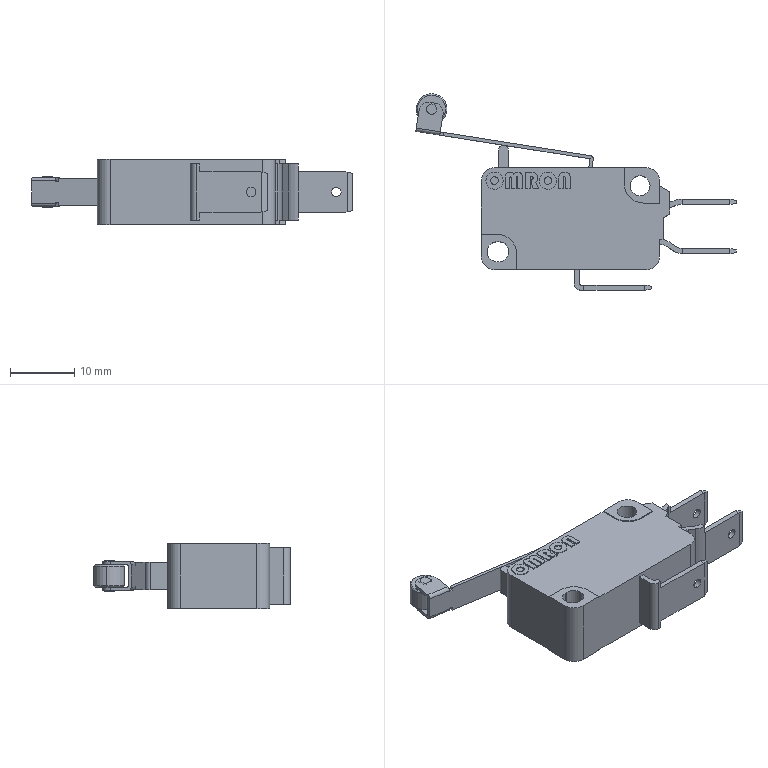Part | SolidWorks | 5 solids | 236 faces | box 50.042 x 30.664 x 10.3 mm | volume 4689 mm3 | plane 143 | cylinder 53 | spline 32 | cone 8 | commonest cylinder face diameters 1 x10 1.5 x9 4 x7 2 x6 3.1 x5 3 x4